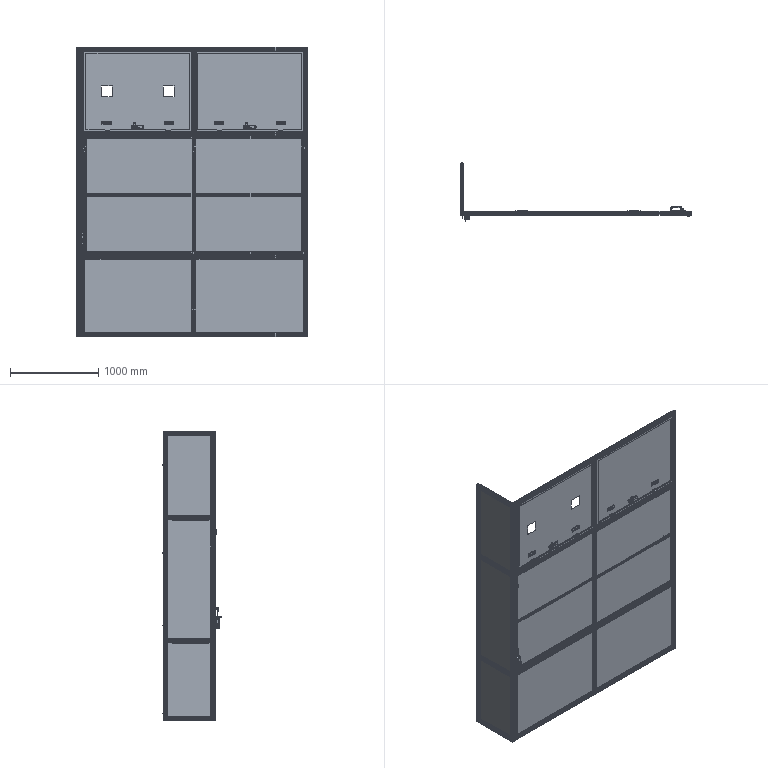Part | SolidWorks | 262 solids | 15308 faces | volume 60412715 mm3 | plane 8561 | cylinder 4277 | cone 1676 | spline 507 | torus 241 | sphere 46 | commonest cylinder face diameters 1 x389 2 x352 6.8 x322 5 x312 2.5 x178 11 x172